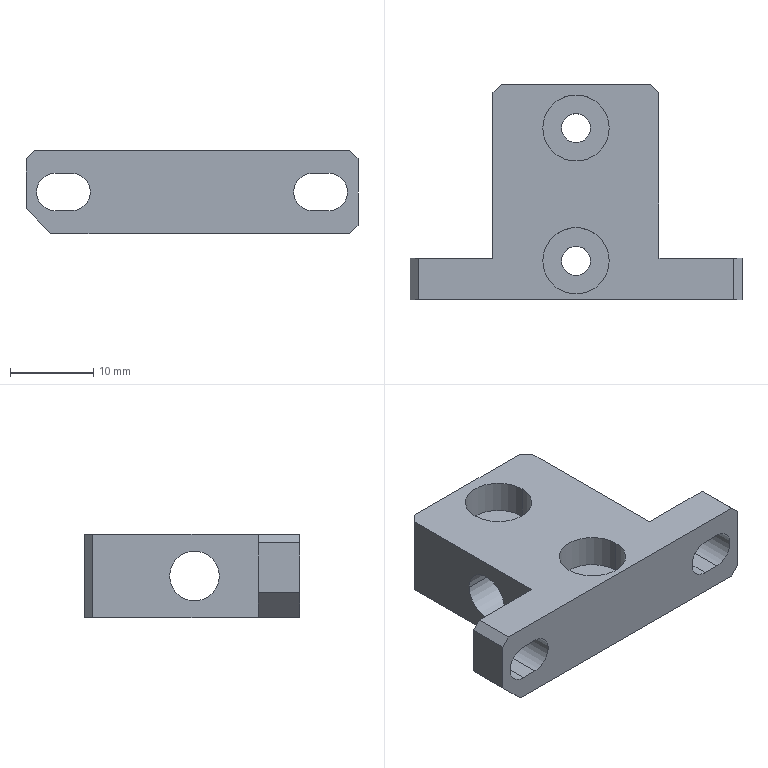Part | SolidWorks | features ICE 3, Chamfer 2, Extrusion 1, HoleWzd 1, MoveFace 1 | 1 solid | 36 faces | box 40 x 26 x 10 mm | volume 4828 mm3 | plane 22 | cylinder 14 | commonest cylinder face diameters 3.5 x4 4.5 x4 8 x4 6 x2
STEP:
#1=CARTESIAN_POINT('',(6.,20.7,6.));
#2=VERTEX_POINT('',#1);
#3=CARTESIAN_POINT('',(14.,20.7,6.));
#4=VERTEX_POINT('',#3);
#5=CARTESIAN_POINT('',(10.,20.7,6.));
#6=DIRECTION('',(0.,0.,1.));
#7=DIRECTION('',(1.,0.,0.));
#8=AXIS2_PLACEMENT_3D('',#5,#6,#7);
#9=CIRCLE('',#8,4.);
#10=EDGE_CURVE('',#2,#4,#9,.T.);
#11=ORIENTED_EDGE('',*,*,#10,.F.);
#12=CARTESIAN_POINT('',(6.,20.7,10.));
#13=VERTEX_POINT('',#12);
#14=CARTESIAN_POINT('',(6.,20.7,10.));
#15=DIRECTION('',(0.,0.,1.));
#16=VECTOR('',#15,1000.);
#17=LINE('',#14,#16);
#18=EDGE_CURVE('',#2,#13,#17,.T.);
#19=ORIENTED_EDGE('',*,*,#18,.T.);
#20=CARTESIAN_POINT('',(14.,20.7,10.));
#21=VERTEX_POINT('',#20);
#22=CARTESIAN_POINT('',(10.,20.7,10.));
#23=DIRECTION('',(0.,0.,1.));
#24=DIRECTION('',(1.,0.,0.));
#25=AXIS2_PLACEMENT_3D('',#22,#23,#24);
#26=CIRCLE('',#25,4.);
#27=EDGE_CURVE('',#13,#21,#26,.T.);
#28=ORIENTED_EDGE('',*,*,#27,.T.);
#29=CARTESIAN_POINT('',(14.,20.7,10.));
#30=DIRECTION('',(0.,0.,1.));
#31=VECTOR('',#30,1000.);
#32=LINE('',#29,#31);
#33=EDGE_CURVE('',#4,#21,#32,.T.);
#34=ORIENTED_EDGE('',*,*,#33,.F.);
#35=EDGE_LOOP('',(#11,#19,#28,#34));
#36=FACE_OUTER_BOUND('',#35,.T.);
#37=CARTESIAN_POINT('',(10.,20.7,10.));
#38=DIRECTION('',(0.,0.,1.));
#39=DIRECTION('',(1.,0.,0.));
#40=AXIS2_PLACEMENT_3D('',#37,#38,#39);
#41=CYLINDRICAL_SURFACE('',#40,4.);
#42=ADVANCED_FACE('',(#36),#41,.F.);
#43=CARTESIAN_POINT('',(11.75,20.7,0.));
#44=VERTEX_POINT('',#43);
#45=CARTESIAN_POINT('',(8.25,20.7,0.));
#46=VERTEX_POINT('',#45);
#47=CARTESIAN_POINT('',(10.,20.7,0.));
#48=DIRECTION('',(0.,0.,-1.));
#49=DIRECTION('',(-1.,0.,0.));
#50=AXIS2_PLACEMENT_3D('',#47,#48,#49);
#51=CIRCLE('',#50,1.75);
#52=EDGE_CURVE('',#44,#46,#51,.T.);
#53=ORIENTED_EDGE('',*,*,#52,.T.);
#54=CARTESIAN_POINT('',(8.25,20.7,6.));
#55=VERTEX_POINT('',#54);
#56=CARTESIAN_POINT('',(8.25,20.7,10.));
#57=DIRECTION('',(0.,0.,1.));
#58=VECTOR('',#57,1000.);
#59=LINE('',#56,#58);
#60=EDGE_CURVE('',#46,#55,#59,.T.);
#61=ORIENTED_EDGE('',*,*,#60,.T.);
#62=CARTESIAN_POINT('',(11.75,20.7,6.));
#63=VERTEX_POINT('',#62);
#64=CARTESIAN_POINT('',(10.,20.7,6.));
#65=DIRECTION('',(0.,0.,1.));
#66=DIRECTION('',(1.,0.,0.));
#67=AXIS2_PLACEMENT_3D('',#64,#65,#66);
#68=CIRCLE('',#67,1.75);
#69=EDGE_CURVE('',#55,#63,#68,.T.);
#70=ORIENTED_EDGE('',*,*,#69,.T.);
#71=CARTESIAN_POINT('',(11.75,20.7,10.));
#72=DIRECTION('',(0.,0.,1.));
#73=VECTOR('',#72,1000.);
#74=LINE('',#71,#73);
#75=EDGE_CURVE('',#44,#63,#74,.T.);
#76=ORIENTED_EDGE('',*,*,#75,.F.);
#77=EDGE_LOOP('',(#53,#61,#70,#76));
#78=FACE_OUTER_BOUND('',#77,.T.);
#79=CARTESIAN_POINT('',(10.,20.7,10.));
#80=DIRECTION('',(0.,0.,1.));
#81=DIRECTION('',(1.,0.,0.));
#82=AXIS2_PLACEMENT_3D('',#79,#80,#81);
#83=CYLINDRICAL_SURFACE('',#82,1.75);
#84=ADVANCED_FACE('',(#78),#83,.F.);
#85=CARTESIAN_POINT('',(6.,4.7,6.));
#86=VERTEX_POINT('',#85);
#87=CARTESIAN_POINT('',(14.,4.7,6.));
#88=VERTEX_POINT('',#87);
#89=CARTESIAN_POINT('',(10.,4.7,6.));
#90=DIRECTION('',(0.,0.,1.));
#91=DIRECTION('',(1.,0.,0.));
#92=AXIS2_PLACEMENT_3D('',#89,#90,#91);
#93=CIRCLE('',#92,4.);
#94=EDGE_CURVE('',#86,#88,#93,.T.);
#95=ORIENTED_EDGE('',*,*,#94,.F.);
#96=CARTESIAN_POINT('',(6.,4.7,10.));
#97=VERTEX_POINT('',#96);
#98=CARTESIAN_POINT('',(6.,4.7,10.));
#99=DIRECTION('',(0.,0.,1.));
#100=VECTOR('',#99,1000.);
#101=LINE('',#98,#100);
#102=EDGE_CURVE('',#86,#97,#101,.T.);
#103=ORIENTED_EDGE('',*,*,#102,.T.);
#104=CARTESIAN_POINT('',(14.,4.7,10.));
#105=VERTEX_POINT('',#104);
#106=CARTESIAN_POINT('',(10.,4.7,10.));
#107=DIRECTION('',(0.,0.,1.));
#108=DIRECTION('',(1.,0.,0.));
#109=AXIS2_PLACEMENT_3D('',#106,#107,#108);
#110=CIRCLE('',#109,4.);
#111=EDGE_CURVE('',#97,#105,#110,.T.);
#112=ORIENTED_EDGE('',*,*,#111,.T.);
#113=CARTESIAN_POINT('',(14.,4.7,10.));
#114=DIRECTION('',(0.,0.,1.));
#115=VECTOR('',#114,1000.);
#116=LINE('',#113,#115);
#117=EDGE_CURVE('',#88,#105,#116,.T.);
#118=ORIENTED_EDGE('',*,*,#117,.F.);
#119=EDGE_LOOP('',(#95,#103,#112,#118));
#120=FACE_OUTER_BOUND('',#119,.T.);
#121=CARTESIAN_POINT('',(10.,4.7,10.));
#122=DIRECTION('',(0.,0.,1.));
#123=DIRECTION('',(1.,0.,0.));
#124=AXIS2_PLACEMENT_3D('',#121,#122,#123);
#125=CYLINDRICAL_SURFACE('',#124,4.);
#126=ADVANCED_FACE('',(#120),#125,.F.);
#127=CARTESIAN_POINT('',(11.75,4.7,0.));
#128=VERTEX_POINT('',#127);
#129=CARTESIAN_POINT('',(8.25,4.7,0.));
#130=VERTEX_POINT('',#129);
#131=CARTESIAN_POINT('',(10.,4.7,0.));
#132=DIRECTION('',(0.,0.,-1.));
#133=DIRECTION('',(-1.,0.,0.));
#134=AXIS2_PLACEMENT_3D('',#131,#132,#133);
#135=CIRCLE('',#134,1.75);
#136=EDGE_CURVE('',#128,#130,#135,.T.);
#137=ORIENTED_EDGE('',*,*,#136,.T.);
#138=CARTESIAN_POINT('',(8.25,4.7,6.));
#139=VERTEX_POINT('',#138);
#140=CARTESIAN_POINT('',(8.25,4.7,10.));
#141=DIRECTION('',(0.,0.,1.));
#142=VECTOR('',#141,1000.);
#143=LINE('',#140,#142);
#144=EDGE_CURVE('',#130,#139,#143,.T.);
#145=ORIENTED_EDGE('',*,*,#144,.T.);
#146=CARTESIAN_POINT('',(11.75,4.7,6.));
#147=VERTEX_POINT('',#146);
#148=CARTESIAN_POINT('',(10.,4.7,6.));
#149=DIRECTION('',(0.,0.,1.));
#150=DIRECTION('',(1.,0.,0.));
#151=AXIS2_PLACEMENT_3D('',#148,#149,#150);
#152=CIRCLE('',#151,1.75);
#153=EDGE_CURVE('',#139,#147,#152,.T.);
#154=ORIENTED_EDGE('',*,*,#153,.T.);
#155=CARTESIAN_POINT('',(11.75,4.7,10.));
#156=DIRECTION('',(0.,0.,1.));
#157=VECTOR('',#156,1000.);
#158=LINE('',#155,#157);
#159=EDGE_CURVE('',#128,#147,#158,.T.);
#160=ORIENTED_EDGE('',*,*,#159,.F.);
#161=EDGE_LOOP('',(#137,#145,#154,#160));
#162=FACE_OUTER_BOUND('',#161,.T.);
#163=CARTESIAN_POINT('',(10.,4.7,10.));
#164=DIRECTION('',(0.,0.,1.));
#165=DIRECTION('',(1.,0.,0.));
#166=AXIS2_PLACEMENT_3D('',#163,#164,#165);
#167=CYLINDRICAL_SURFACE('',#166,1.75);
#168=ADVANCED_FACE('',(#162),#167,.F.);
#169=CARTESIAN_POINT('',(20.,15.7,5.));
#170=VERTEX_POINT('',#169);
#171=CARTESIAN_POINT('',(20.,9.7,5.));
#172=VERTEX_POINT('',#171);
#173=CARTESIAN_POINT('',(20.,12.7,5.));
#174=DIRECTION('',(-1.,0.,0.));
#175=DIRECTION('',(0.,-1.,0.));
#176=AXIS2_PLACEMENT_3D('',#173,#174,#175);
#177=CIRCLE('',#176,3.);
#178=EDGE_CURVE('',#170,#172,#177,.T.);
#179=ORIENTED_EDGE('',*,*,#178,.F.);
#180=CARTESIAN_POINT('',(0.,15.7,5.));
#181=VERTEX_POINT('',#180);
#182=CARTESIAN_POINT('',(30.,15.7,5.));
#183=DIRECTION('',(-1.,0.,0.));
#184=VECTOR('',#183,1000.);
#185=LINE('',#182,#184);
#186=EDGE_CURVE('',#170,#181,#185,.T.);
#187=ORIENTED_EDGE('',*,*,#186,.T.);
#188=CARTESIAN_POINT('',(0.,9.7,5.));
#189=VERTEX_POINT('',#188);
#190=CARTESIAN_POINT('',(0.,12.7,5.));
#191=DIRECTION('',(1.,0.,0.));
#192=DIRECTION('',(0.,0.,-1.));
#193=AXIS2_PLACEMENT_3D('',#190,#191,#192);
#194=CIRCLE('',#193,3.);
#195=EDGE_CURVE('',#189,#181,#194,.T.);
#196=ORIENTED_EDGE('',*,*,#195,.F.);
#197=CARTESIAN_POINT('',(30.,9.7,5.));
#198=DIRECTION('',(-1.,0.,0.));
#199=VECTOR('',#198,1000.);
#200=LINE('',#197,#199);
#201=EDGE_CURVE('',#172,#189,#200,.T.);
#202=ORIENTED_EDGE('',*,*,#201,.F.);
#203=EDGE_LOOP('',(#179,#187,#196,#202));
#204=FACE_OUTER_BOUND('',#203,.T.);
#205=CARTESIAN_POINT('',(30.,12.7,5.));
#206=DIRECTION('',(-1.,0.,0.));
#207=DIRECTION('',(0.,-1.,0.));
#208=AXIS2_PLACEMENT_3D('',#205,#206,#207);
#209=CYLINDRICAL_SURFACE('',#208,3.);
#210=ADVANCED_FACE('',(#204),#209,.F.);
#211=ORIENTED_EDGE('',*,*,#195,.T.);
#212=CARTESIAN_POINT('',(0.,12.7,5.));
#213=DIRECTION('',(1.,0.,0.));
#214=DIRECTION('',(0.,0.,-1.));
#215=AXIS2_PLACEMENT_3D('',#212,#213,#214);
#216=CIRCLE('',#215,3.);
#217=EDGE_CURVE('',#181,#189,#216,.T.);
#218=ORIENTED_EDGE('',*,*,#217,.T.);
#219=EDGE_LOOP('',(#211,#218));
#220=FACE_BOUND('',#219,.T.);
#221=CARTESIAN_POINT('',(0.,25.,10.));
#222=VERTEX_POINT('',#221);
#223=CARTESIAN_POINT('',(0.,5.,10.));
#224=VERTEX_POINT('',#223);
#225=CARTESIAN_POINT('',(0.,0.,10.));
#226=DIRECTION('',(0.,-1.,0.));
#227=VECTOR('',#226,1000.);
#228=LINE('',#225,#227);
#229=EDGE_CURVE('',#222,#224,#228,.T.);
#230=ORIENTED_EDGE('',*,*,#229,.F.);
#231=CARTESIAN_POINT('',(0.,25.,0.));
#232=VERTEX_POINT('',#231);
#233=CARTESIAN_POINT('',(0.,25.,10.));
#234=DIRECTION('',(0.,0.,-1.));
#235=VECTOR('',#234,1000.);
#236=LINE('',#233,#235);
#237=EDGE_CURVE('',#222,#232,#236,.T.);
#238=ORIENTED_EDGE('',*,*,#237,.T.);
#239=CARTESIAN_POINT('',(0.,5.,0.));
#240=VERTEX_POINT('',#239);
#241=CARTESIAN_POINT('',(0.,0.,0.));
#242=DIRECTION('',(0.,-1.,0.));
#243=VECTOR('',#242,1000.);
#244=LINE('',#241,#243);
#245=EDGE_CURVE('',#232,#240,#244,.T.);
#246=ORIENTED_EDGE('',*,*,#245,.T.);
#247=CARTESIAN_POINT('',(0.,5.,10.));
#248=DIRECTION('',(0.,0.,1.));
#249=VECTOR('',#248,1000.);
#250=LINE('',#247,#249);
#251=EDGE_CURVE('',#240,#224,#250,.T.);
#252=ORIENTED_EDGE('',*,*,#251,.T.);
#253=EDGE_LOOP('',(#230,#238,#246,#252));
#254=FACE_OUTER_BOUND('',#253,.T.);
#255=CARTESIAN_POINT('',(0.,0.,10.));
#256=DIRECTION('',(1.,0.,0.));
#257=DIRECTION('',(0.,0.,-1.));
#258=AXIS2_PLACEMENT_3D('',#255,#256,#257);
#259=PLANE('',#258);
#260=ADVANCED_FACE('',(#220,#254),#259,.F.);
#261=CARTESIAN_POINT('',(-4.5,0.,2.75));
#262=VERTEX_POINT('',#261);
#263=CARTESIAN_POINT('',(-6.5,0.,2.75));
#264=VERTEX_POINT('',#263);
#265=CARTESIAN_POINT('',(-6.5,0.,2.75));
#266=DIRECTION('',(-1.,0.,0.));
#267=VECTOR('',#266,1000.);
#268=LINE('',#265,#267);
#269=EDGE_CURVE('',#262,#264,#268,.T.);
#270=ORIENTED_EDGE('',*,*,#269,.T.);
#271=CARTESIAN_POINT('',(-6.5,0.,7.25));
#272=VERTEX_POINT('',#271);
#273=CARTESIAN_POINT('',(-6.5,0.,5.));
#274=DIRECTION('',(0.,1.,0.));
#275=DIRECTION('',(0.,0.,1.));
#276=AXIS2_PLACEMENT_3D('',#273,#274,#275);
#277=CIRCLE('',#276,2.25);
#278=EDGE_CURVE('',#264,#272,#277,.T.);
#279=ORIENTED_EDGE('',*,*,#278,.T.);
#280=CARTESIAN_POINT('',(-4.5,0.,7.25));
#281=VERTEX_POINT('',#280);
#282=CARTESIAN_POINT('',(-6.5,0.,7.25));
#283=DIRECTION('',(1.,0.,0.));
#284=VECTOR('',#283,1000.);
#285=LINE('',#282,#284);
#286=EDGE_CURVE('',#272,#281,#285,.T.);
#287=ORIENTED_EDGE('',*,*,#286,.T.);
#288=CARTESIAN_POINT('',(-4.5,0.,5.));
#289=DIRECTION('',(0.,1.,0.));
#290=DIRECTION('',(0.,0.,1.));
#291=AXIS2_PLACEMENT_3D('',#288,#289,#290);
#292=CIRCLE('',#291,2.25);
#293=EDGE_CURVE('',#281,#262,#292,.T.);
#294=ORIENTED_EDGE('',*,*,#293,.T.);
#295=EDGE_LOOP('',(#270,#279,#287,#294));
#296=FACE_BOUND('',#295,.T.);
#297=CARTESIAN_POINT('',(24.5,0.,7.25));
#298=VERTEX_POINT('',#297);
#299=CARTESIAN_POINT('',(26.5,0.,7.25));
#300=VERTEX_POINT('',#299);
#301=CARTESIAN_POINT('',(26.5,0.,7.25));
#302=DIRECTION('',(1.,0.,0.));
#303=VECTOR('',#302,1000.);
#304=LINE('',#301,#303);
#305=EDGE_CURVE('',#298,#300,#304,.T.);
#306=ORIENTED_EDGE('',*,*,#305,.T.);
#307=CARTESIAN_POINT('',(26.5,0.,2.75));
#308=VERTEX_POINT('',#307);
#309=CARTESIAN_POINT('',(26.5,0.,5.));
#310=DIRECTION('',(0.,1.,0.));
#311=DIRECTION('',(0.,0.,-1.));
#312=AXIS2_PLACEMENT_3D('',#309,#310,#311);
#313=CIRCLE('',#312,2.25);
#314=EDGE_CURVE('',#300,#308,#313,.T.);
#315=ORIENTED_EDGE('',*,*,#314,.T.);
#316=CARTESIAN_POINT('',(24.5,0.,2.75));
#317=VERTEX_POINT('',#316);
#318=CARTESIAN_POINT('',(26.5,0.,2.75));
#319=DIRECTION('',(-1.,0.,0.));
#320=VECTOR('',#319,1000.);
#321=LINE('',#318,#320);
#322=EDGE_CURVE('',#308,#317,#321,.T.);
#323=ORIENTED_EDGE('',*,*,#322,.T.);
#324=CARTESIAN_POINT('',(24.5,0.,5.));
#325=DIRECTION('',(0.,1.,0.));
#326=DIRECTION('',(0.,0.,-1.));
#327=AXIS2_PLACEMENT_3D('',#324,#325,#326);
#328=CIRCLE('',#327,2.25);
#329=EDGE_CURVE('',#317,#298,#328,.T.);
#330=ORIENTED_EDGE('',*,*,#329,.T.);
#331=EDGE_LOOP('',(#306,#315,#323,#330));
#332=FACE_BOUND('',#331,.T.);
#333=CARTESIAN_POINT('',(-10.,0.,9.));
#334=VERTEX_POINT('',#333);
#335=CARTESIAN_POINT('',(-10.,0.,3.));
#336=VERTEX_POINT('',#335);
#337=CARTESIAN_POINT('',(-10.,0.,10.));
#338=DIRECTION('',(0.,0.,-1.));
#339=VECTOR('',#338,1000.);
#340=LINE('',#337,#339);
#341=EDGE_CURVE('',#334,#336,#340,.T.);
#342=ORIENTED_EDGE('',*,*,#341,.T.);
#343=CARTESIAN_POINT('',(-7.,0.,0.));
#344=VERTEX_POINT('',#343);
#345=CARTESIAN_POINT('',(-10.,0.,3.));
#346=DIRECTION('',(0.7071,0.,-0.7071));
#347=VECTOR('',#346,1000.);
#348=LINE('',#345,#347);
#349=EDGE_CURVE('',#336,#344,#348,.T.);
#350=ORIENTED_EDGE('',*,*,#349,.T.);
#351=CARTESIAN_POINT('',(29.,0.,0.));
#352=VERTEX_POINT('',#351);
#353=CARTESIAN_POINT('',(0.,0.,0.));
#354=DIRECTION('',(1.,0.,0.));
#355=VECTOR('',#354,1000.);
#356=LINE('',#353,#355);
#357=EDGE_CURVE('',#344,#352,#356,.T.);
#358=ORIENTED_EDGE('',*,*,#357,.T.);
#359=CARTESIAN_POINT('',(30.,0.,1.));
#360=VERTEX_POINT('',#359);
#361=CARTESIAN_POINT('',(29.,0.,0.));
#362=DIRECTION('',(0.7071,0.,0.7071));
#363=VECTOR('',#362,1000.);
#364=LINE('',#361,#363);
#365=EDGE_CURVE('',#352,#360,#364,.T.);
#366=ORIENTED_EDGE('',*,*,#365,.T.);
#367=CARTESIAN_POINT('',(30.,0.,9.));
#368=VERTEX_POINT('',#367);
#369=CARTESIAN_POINT('',(30.,0.,10.));
#370=DIRECTION('',(0.,0.,1.));
#371=VECTOR('',#370,1000.);
#372=LINE('',#369,#371);
#373=EDGE_CURVE('',#360,#368,#372,.T.);
#374=ORIENTED_EDGE('',*,*,#373,.T.);
#375=CARTESIAN_POINT('',(29.,0.,10.));
#376=VERTEX_POINT('',#375);
#377=CARTESIAN_POINT('',(30.,0.,9.));
#378=DIRECTION('',(-0.7071,0.,0.7071));
#379=VECTOR('',#378,1000.);
#380=LINE('',#377,#379);
#381=EDGE_CURVE('',#368,#376,#380,.T.);
#382=ORIENTED_EDGE('',*,*,#381,.T.);
#383=CARTESIAN_POINT('',(-9.,0.,10.));
#384=VERTEX_POINT('',#383);
#385=CARTESIAN_POINT('',(0.,0.,10.));
#386=DIRECTION('',(1.,0.,0.));
#387=VECTOR('',#386,1000.);
#388=LINE('',#385,#387);
#389=EDGE_CURVE('',#384,#376,#388,.T.);
#390=ORIENTED_EDGE('',*,*,#389,.F.);
#391=CARTESIAN_POINT('',(-9.,0.,10.));
#392=DIRECTION('',(-0.7071,0.,-0.7071));
#393=VECTOR('',#392,1000.);
#394=LINE('',#391,#393);
#395=EDGE_CURVE('',#384,#334,#394,.T.);
#396=ORIENTED_EDGE('',*,*,#395,.T.);
#397=EDGE_LOOP('',(#342,#350,#358,#366,#374,#382,#390,#396));
#398=FACE_OUTER_BOUND('',#397,.T.);
#399=CARTESIAN_POINT('',(0.,0.,10.));
#400=DIRECTION('',(0.,1.,0.));
#401=DIRECTION('',(0.,0.,1.));
#402=AXIS2_PLACEMENT_3D('',#399,#400,#401);
#403=PLANE('',#402);
#404=ADVANCED_FACE('',(#296,#332,#398),#403,.F.);
#405=CARTESIAN_POINT('',(20.,12.7,5.));
#406=DIRECTION('',(-1.,0.,0.));
#407=DIRECTION('',(0.,-1.,0.));
#408=AXIS2_PLACEMENT_3D('',#405,#406,#407);
#409=CIRCLE('',#408,3.);
#410=EDGE_CURVE('',#172,#170,#409,.T.);
#411=ORIENTED_EDGE('',*,*,#410,.T.);
#412=ORIENTED_EDGE('',*,*,#178,.T.);
#413=EDGE_LOOP('',(#411,#412));
#414=FACE_BOUND('',#413,.T.);
#415=CARTESIAN_POINT('',(20.,5.,0.));
#416=VERTEX_POINT('',#415);
#417=CARTESIAN_POINT('',(20.,25.,0.));
#418=VERTEX_POINT('',#417);
#419=CARTESIAN_POINT('',(20.,0.,0.));
#420=DIRECTION('',(0.,1.,0.));
#421=VECTOR('',#420,1000.);
#422=LINE('',#419,#421);
#423=EDGE_CURVE('',#416,#418,#422,.T.);
#424=ORIENTED_EDGE('',*,*,#423,.T.);
#425=CARTESIAN_POINT('',(20.,25.,10.));
#426=VERTEX_POINT('',#425);
#427=CARTESIAN_POINT('',(20.,25.,10.));
#428=DIRECTION('',(0.,0.,1.));
#429=VECTOR('',#428,1000.);
#430=LINE('',#427,#429);
#431=EDGE_CURVE('',#418,#426,#430,.T.);
#432=ORIENTED_EDGE('',*,*,#431,.T.);
#433=CARTESIAN_POINT('',(20.,5.,10.));
#434=VERTEX_POINT('',#433);
#435=CARTESIAN_POINT('',(20.,0.,10.));
#436=DIRECTION('',(0.,1.,0.));
#437=VECTOR('',#436,1000.);
#438=LINE('',#435,#437);
#439=EDGE_CURVE('',#434,#426,#438,.T.);
#440=ORIENTED_EDGE('',*,*,#439,.F.);
#441=CARTESIAN_POINT('',(20.,5.,10.));
#442=DIRECTION('',(0.,0.,-1.));
#443=VECTOR('',#442,1000.);
#444=LINE('',#441,#443);
#445=EDGE_CURVE('',#434,#416,#444,.T.);
#446=ORIENTED_EDGE('',*,*,#445,.T.);
#447=EDGE_LOOP('',(#424,#432,#440,#446));
#448=FACE_OUTER_BOUND('',#447,.T.);
#449=CARTESIAN_POINT('',(20.,0.,10.));
#450=DIRECTION('',(-1.,0.,0.));
#451=DIRECTION('',(0.,-1.,0.));
#452=AXIS2_PLACEMENT_3D('',#449,#450,#451);
#453=PLANE('',#452);
#454=ADVANCED_FACE('',(#414,#448),#453,.F.);
#455=CARTESIAN_POINT('',(19.,26.,10.));
#456=VERTEX_POINT('',#455);
#457=CARTESIAN_POINT('',(1.,26.,10.));
#458=VERTEX_POINT('',#457);
#459=CARTESIAN_POINT('',(0.,26.,10.));
#460=DIRECTION('',(-1.,0.,0.));
#461=VECTOR('',#460,1000.);
#462=LINE('',#459,#461);
#463=EDGE_CURVE('',#456,#458,#462,.T.);
#464=ORIENTED_EDGE('',*,*,#463,.F.);
#465=CARTESIAN_POINT('',(19.,26.,0.));
#466=VERTEX_POINT('',#465);
#467=CARTESIAN_POINT('',(19.,26.,10.));
#468=DIRECTION('',(0.,0.,-1.));
#469=VECTOR('',#468,1000.);
#470=LINE('',#467,#469);
#471=EDGE_CURVE('',#456,#466,#470,.T.);
#472=ORIENTED_EDGE('',*,*,#471,.T.);
#473=CARTESIAN_POINT('',(1.,26.,0.));
#474=VERTEX_POINT('',#473);
#475=CARTESIAN_POINT('',(0.,26.,0.));
#476=DIRECTION('',(-1.,0.,0.));
#477=VECTOR('',#476,1000.);
#478=LINE('',#475,#477);
#479=EDGE_CURVE('',#466,#474,#478,.T.);
#480=ORIENTED_EDGE('',*,*,#479,.T.);
#481=CARTESIAN_POINT('',(1.,26.,10.));
#482=DIRECTION('',(0.,0.,1.));
#483=VECTOR('',#482,1000.);
#484=LINE('',#481,#483);
#485=EDGE_CURVE('',#474,#458,#484,.T.);
#486=ORIENTED_EDGE('',*,*,#485,.T.);
#487=EDGE_LOOP('',(#464,#472,#480,#486));
#488=FACE_OUTER_BOUND('',#487,.T.);
#489=CARTESIAN_POINT('',(0.,26.,10.));
#490=DIRECTION('',(0.,-1.,0.));
#491=DIRECTION('',(0.,0.,-1.));
#492=AXIS2_PLACEMENT_3D('',#489,#490,#491);
#493=PLANE('',#492);
#494=ADVANCED_FACE('',(#488),#493,.F.);
#495=CARTESIAN_POINT('',(10.,20.7,10.));
#496=DIRECTION('',(0.,0.,1.));
#497=DIRECTION('',(1.,0.,0.));
#498=AXIS2_PLACEMENT_3D('',#495,#496,#497);
#499=CIRCLE('',#498,4.);
#500=EDGE_CURVE('',#21,#13,#499,.T.);
#501=ORIENTED_EDGE('',*,*,#500,.F.);
#502=ORIENTED_EDGE('',*,*,#27,.F.);
#503=EDGE_LOOP('',(#501,#502));
#504=FACE_BOUND('',#503,.T.);
#505=CARTESIAN_POINT('',(10.,4.7,10.));
#506=DIRECTION('',(0.,0.,1.));
#507=DIRECTION('',(1.,0.,0.));
#508=AXIS2_PLACEMENT_3D('',#505,#506,#507);
#509=CIRCLE('',#508,4.);
#510=EDGE_CURVE('',#105,#97,#509,.T.);
#511=ORIENTED_EDGE('',*,*,#510,.F.);
#512=ORIENTED_EDGE('',*,*,#111,.F.);
#513=EDGE_LOOP('',(#511,#512));
#514=FACE_BOUND('',#513,.T.);
#515=ORIENTED_EDGE('',*,*,#389,.T.);
#516=CARTESIAN_POINT('',(29.,5.,10.));
#517=VERTEX_POINT('',#516);
#518=CARTESIAN_POINT('',(29.,8.,10.));
#519=DIRECTION('',(0.,1.,0.));
#520=VECTOR('',#519,1000.);
#521=LINE('',#518,#520);
#522=EDGE_CURVE('',#376,#517,#521,.T.);
#523=ORIENTED_EDGE('',*,*,#522,.T.);
#524=CARTESIAN_POINT('',(-10.,5.,10.));
#525=DIRECTION('',(-1.,0.,0.));
#526=VECTOR('',#525,1000.);
#527=LINE('',#524,#526);
#528=EDGE_CURVE('',#517,#434,#527,.T.);
#529=ORIENTED_EDGE('',*,*,#528,.T.);
#530=ORIENTED_EDGE('',*,*,#439,.T.);
#531=CARTESIAN_POINT('',(19.,26.,10.));
#532=DIRECTION('',(-0.7071,0.7071,0.));
#533=VECTOR('',#532,1000.);
#534=LINE('',#531,#533);
#535=EDGE_CURVE('',#426,#456,#534,.T.);
#536=ORIENTED_EDGE('',*,*,#535,.T.);
#537=ORIENTED_EDGE('',*,*,#463,.T.);
#538=CARTESIAN_POINT('',(0.,25.,10.));
#539=DIRECTION('',(-0.7071,-0.7071,0.));
#540=VECTOR('',#539,1000.);
#541=LINE('',#538,#540);
#542=EDGE_CURVE('',#458,#222,#541,.T.);
#543=ORIENTED_EDGE('',*,*,#542,.T.);
#544=ORIENTED_EDGE('',*,*,#229,.T.);
#545=CARTESIAN_POINT('',(-9.,5.,10.));
#546=VERTEX_POINT('',#545);
#547=CARTESIAN_POINT('',(-10.,5.,10.));
#548=DIRECTION('',(-1.,0.,0.));
#549=VECTOR('',#548,1000.);
#550=LINE('',#547,#549);
#551=EDGE_CURVE('',#224,#546,#550,.T.);
#552=ORIENTED_EDGE('',*,*,#551,.T.);
#553=CARTESIAN_POINT('',(-9.,0.,10.));
#554=DIRECTION('',(0.,-1.,0.));
#555=VECTOR('',#554,1000.);
#556=LINE('',#553,#555);
#557=EDGE_CURVE('',#546,#384,#556,.T.);
#558=ORIENTED_EDGE('',*,*,#557,.T.);
#559=EDGE_LOOP('',(#515,#523,#529,#530,#536,#537,#543,#544,#552,#558));
#560=FACE_OUTER_BOUND('',#559,.T.);
#561=CARTESIAN_POINT('',(0.,0.,10.));
#562=DIRECTION('',(0.,0.,-1.));
#563=DIRECTION('',(-1.,0.,0.));
#564=AXIS2_PLACEMENT_3D('',#561,#562,#563);
#565=PLANE('',#564);
#566=ADVANCED_FACE('',(#504,#514,#560),#565,.F.);
#567=ORIENTED_EDGE('',*,*,#52,.F.);
#568=CARTESIAN_POINT('',(10.,20.7,0.));
#569=DIRECTION('',(0.,0.,-1.));
#570=DIRECTION('',(-1.,0.,0.));
#571=AXIS2_PLACEMENT_3D('',#568,#569,#570);
#572=CIRCLE('',#571,1.75);
#573=EDGE_CURVE('',#46,#44,#572,.T.);
#574=ORIENTED_EDGE('',*,*,#573,.F.);
#575=EDGE_LOOP('',(#567,#574));
#576=FACE_BOUND('',#575,.T.);
#577=ORIENTED_EDGE('',*,*,#136,.F.);
#578=CARTESIAN_POINT('',(10.,4.7,0.));
#579=DIRECTION('',(0.,0.,-1.));
#580=DIRECTION('',(-1.,0.,0.));
#581=AXIS2_PLACEMENT_3D('',#578,#579,#580);
#582=CIRCLE('',#581,1.75);
#583=EDGE_CURVE('',#130,#128,#582,.T.);
#584=ORIENTED_EDGE('',*,*,#583,.F.);
#585=EDGE_LOOP('',(#577,#584));
#586=FACE_BOUND('',#585,.T.);
#587=ORIENTED_EDGE('',*,*,#357,.F.);
#588=CARTESIAN_POINT('',(-7.,5.,0.));
#589=VERTEX_POINT('',#588);
#590=CARTESIAN_POINT('',(-7.,0.,0.));
#591=DIRECTION('',(0.,1.,0.));
#592=VECTOR('',#591,1000.);
#593=LINE('',#590,#592);
#594=EDGE_CURVE('',#344,#589,#593,.T.);
#595=ORIENTED_EDGE('',*,*,#594,.T.);
#596=CARTESIAN_POINT('',(-10.,5.,0.));
#597=DIRECTION('',(1.,0.,0.));
#598=VECTOR('',#597,1000.);
#599=LINE('',#596,#598);
#600=EDGE_CURVE('',#589,#240,#599,.T.);
#601=ORIENTED_EDGE('',*,*,#600,.T.);
#602=ORIENTED_EDGE('',*,*,#245,.F.);
#603=CARTESIAN_POINT('',(-12.5,12.5,0.));
#604=DIRECTION('',(0.7071,0.7071,0.));
#605=VECTOR('',#604,1000.);
#606=LINE('',#603,#605);
#607=EDGE_CURVE('',#232,#474,#606,.T.);
#608=ORIENTED_EDGE('',*,*,#607,.T.);
#609=ORIENTED_EDGE('',*,*,#479,.F.);
#610=CARTESIAN_POINT('',(22.5,22.5,0.));
#611=DIRECTION('',(0.7071,-0.7071,0.));
#612=VECTOR('',#611,1000.);
#613=LINE('',#610,#612);
#614=EDGE_CURVE('',#466,#418,#613,.T.);
#615=ORIENTED_EDGE('',*,*,#614,.T.);
#616=ORIENTED_EDGE('',*,*,#423,.F.);
#617=CARTESIAN_POINT('',(29.,5.,0.));
#618=VERTEX_POINT('',#617);
#619=CARTESIAN_POINT('',(-10.,5.,0.));
#620=DIRECTION('',(1.,0.,0.));
#621=VECTOR('',#620,1000.);
#622=LINE('',#619,#621);
#623=EDGE_CURVE('',#416,#618,#622,.T.);
#624=ORIENTED_EDGE('',*,*,#623,.T.);
#625=CARTESIAN_POINT('',(29.,0.,0.));
#626=DIRECTION('',(0.,-1.,0.));
#627=VECTOR('',#626,1000.);
#628=LINE('',#625,#627);
#629=EDGE_CURVE('',#618,#352,#628,.T.);
#630=ORIENTED_EDGE('',*,*,#629,.T.);
#631=EDGE_LOOP('',(#587,#595,#601,#602,#608,#609,#615,#616,#624,#630));
#632=FACE_OUTER_BOUND('',#631,.T.);
#633=CARTESIAN_POINT('',(0.,0.,0.));
#634=DIRECTION('',(0.,0.,-1.));
#635=DIRECTION('',(-1.,0.,0.));
#636=AXIS2_PLACEMENT_3D('',#633,#634,#635);
#637=PLANE('',#636);
#638=ADVANCED_FACE('',(#576,#586,#632),#637,.T.);
#639=ORIENTED_EDGE('',*,*,#373,.F.);
#640=CARTESIAN_POINT('',(30.,5.,1.));
#641=VERTEX_POINT('',#640);
#642=CARTESIAN_POINT('',(30.,8.,1.));
#643=DIRECTION('',(0.,1.,0.));
#644=VECTOR('',#643,1000.);
#645=LINE('',#642,#644);
#646=EDGE_CURVE('',#360,#641,#645,.T.);
#647=ORIENTED_EDGE('',*,*,#646,.T.);
#648=CARTESIAN_POINT('',(30.,5.,9.));
#649=VERTEX_POINT('',#648);
#650=CARTESIAN_POINT('',(30.,5.,10.));
#651=DIRECTION('',(0.,0.,1.));
#652=VECTOR('',#651,1000.);
#653=LINE('',#650,#652);
#654=EDGE_CURVE('',#641,#649,#653,.T.);
#655=ORIENTED_EDGE('',*,*,#654,.T.);
#656=CARTESIAN_POINT('',(30.,0.,9.));
#657=DIRECTION('',(0.,-1.,0.));
#658=VECTOR('',#657,1000.);
#659=LINE('',#656,#658);
#660=EDGE_CURVE('',#649,#368,#659,.T.);
#661=ORIENTED_EDGE('',*,*,#660,.T.);
#662=EDGE_LOOP('',(#639,#647,#655,#661));
#663=FACE_OUTER_BOUND('',#662,.T.);
#664=CARTESIAN_POINT('',(30.,8.,10.));
#665=DIRECTION('',(1.,0.,0.));
#666=DIRECTION('',(0.,0.,-1.));
#667=AXIS2_PLACEMENT_3D('',#664,#665,#666);
#668=PLANE('',#667);
#669=ADVANCED_FACE('',(#663),#668,.T.);
#670=CARTESIAN_POINT('',(26.5,5.,7.25));
#671=VERTEX_POINT('',#670);
#672=CARTESIAN_POINT('',(26.5,5.,2.75));
#673=VERTEX_POINT('',#672);
#674=CARTESIAN_POINT('',(26.5,5.,5.));
#675=DIRECTION('',(0.,1.,0.));
#676=DIRECTION('',(0.,0.,-1.));
#677=AXIS2_PLACEMENT_3D('',#674,#675,#676);
#678=CIRCLE('',#677,2.25);
#679=EDGE_CURVE('',#671,#673,#678,.T.);
#680=ORIENTED_EDGE('',*,*,#679,.F.);
#681=CARTESIAN_POINT('',(24.5,5.,7.25));
#682=VERTEX_POINT('',#681);
#683=CARTESIAN_POINT('',(26.5,5.,7.25));
#684=DIRECTION('',(1.,0.,0.));
#685=VECTOR('',#684,1000.);
#686=LINE('',#683,#685);
#687=EDGE_CURVE('',#682,#671,#686,.T.);
#688=ORIENTED_EDGE('',*,*,#687,.F.);
#689=CARTESIAN_POINT('',(24.5,5.,2.75));
#690=VERTEX_POINT('',#689);
#691=CARTESIAN_POINT('',(24.5,5.,5.));
#692=DIRECTION('',(0.,1.,0.));
#693=DIRECTION('',(0.,0.,-1.));
#694=AXIS2_PLACEMENT_3D('',#691,#692,#693);
#695=CIRCLE('',#694,2.25);
#696=EDGE_CURVE('',#690,#682,#695,.T.);
#697=ORIENTED_EDGE('',*,*,#696,.F.);
#698=CARTESIAN_POINT('',(26.5,5.,2.75));
#699=DIRECTION('',(-1.,0.,0.));
#700=VECTOR('',#699,1000.);
#701=LINE('',#698,#700);
#702=EDGE_CURVE('',#673,#690,#701,.T.);
#703=ORIENTED_EDGE('',*,*,#702,.F.);
#704=EDGE_LOOP('',(#680,#688,#697,#703));
#705=FACE_BOUND('',#704,.T.);
#706=ORIENTED_EDGE('',*,*,#654,.F.);
#707=CARTESIAN_POINT('',(14.5,5.,-14.5));
#708=DIRECTION('',(-0.7071,0.,-0.7071));
#709=VECTOR('',#708,1000.);
#710=LINE('',#707,#709);
#711=EDGE_CURVE('',#641,#618,#710,.T.);
#712=ORIENTED_EDGE('',*,*,#711,.T.);
#713=ORIENTED_EDGE('',*,*,#623,.F.);
#714=ORIENTED_EDGE('',*,*,#445,.F.);
#715=ORIENTED_EDGE('',*,*,#528,.F.);
#716=CARTESIAN_POINT('',(19.5,5.,19.5));
#717=DIRECTION('',(0.7071,0.,-0.7071));
#718=VECTOR('',#717,1000.);
#719=LINE('',#716,#718);
#720=EDGE_CURVE('',#517,#649,#719,.T.);
#721=ORIENTED_EDGE('',*,*,#720,.T.);
#722=EDGE_LOOP('',(#706,#712,#713,#714,#715,#721));
#723=FACE_OUTER_BOUND('',#722,.T.);
#724=CARTESIAN_POINT('',(0.,5.,0.));
#725=DIRECTION('',(0.,1.,0.));
#726=DIRECTION('',(0.,0.,1.));
#727=AXIS2_PLACEMENT_3D('',#724,#725,#726);
#728=PLANE('',#727);
#729=ADVANCED_FACE('',(#705,#723),#728,.T.);
#730=CARTESIAN_POINT('',(-6.5,5.,2.75));
#731=VERTEX_POINT('',#730);
#732=CARTESIAN_POINT('',(-6.5,5.,7.25));
#733=VERTEX_POINT('',#732);
#734=CARTESIAN_POINT('',(-6.5,5.,5.));
#735=DIRECTION('',(0.,1.,0.));
#736=DIRECTION('',(0.,0.,1.));
#737=AXIS2_PLACEMENT_3D('',#734,#735,#736);
#738=CIRCLE('',#737,2.25);
#739=EDGE_CURVE('',#731,#733,#738,.T.);
#740=ORIENTED_EDGE('',*,*,#739,.F.);
#741=CARTESIAN_POINT('',(-4.5,5.,2.75));
#742=VERTEX_POINT('',#741);
#743=CARTESIAN_POINT('',(-6.5,5.,2.75));
#744=DIRECTION('',(-1.,0.,0.));
#745=VECTOR('',#744,1000.);
#746=LINE('',#743,#745);
#747=EDGE_CURVE('',#742,#731,#746,.T.);
#748=ORIENTED_EDGE('',*,*,#747,.F.);
#749=CARTESIAN_POINT('',(-4.5,5.,7.25));
#750=VERTEX_POINT('',#749);
#751=CARTESIAN_POINT('',(-4.5,5.,5.));
#752=DIRECTION('',(0.,1.,0.));
#753=DIRECTION('',(0.,0.,1.));
#754=AXIS2_PLACEMENT_3D('',#751,#752,#753);
#755=CIRCLE('',#754,2.25);
#756=EDGE_CURVE('',#750,#742,#755,.T.);
#757=ORIENTED_EDGE('',*,*,#756,.F.);
#758=CARTESIAN_POINT('',(-6.5,5.,7.25));
#759=DIRECTION('',(1.,0.,0.));
#760=VECTOR('',#759,1000.);
#761=LINE('',#758,#760);
#762=EDGE_CURVE('',#733,#750,#761,.T.);
#763=ORIENTED_EDGE('',*,*,#762,.F.);
#764=EDGE_LOOP('',(#740,#748,#757,#763));
#765=FACE_BOUND('',#764,.T.);
#766=ORIENTED_EDGE('',*,*,#600,.F.);
#767=CARTESIAN_POINT('',(-10.,5.,3.));
#768=VERTEX_POINT('',#767);
#769=CARTESIAN_POINT('',(-3.5,5.,-3.5));
#770=DIRECTION('',(-0.7071,0.,0.7071));
#771=VECTOR('',#770,1000.);
#772=LINE('',#769,#771);
#773=EDGE_CURVE('',#589,#768,#772,.T.);
#774=ORIENTED_EDGE('',*,*,#773,.T.);
#775=CARTESIAN_POINT('',(-10.,5.,9.));
#776=VERTEX_POINT('',#775);
#777=CARTESIAN_POINT('',(-10.,5.,10.));
#778=DIRECTION('',(0.,0.,-1.));
#779=VECTOR('',#778,1000.);
#780=LINE('',#777,#779);
#781=EDGE_CURVE('',#776,#768,#780,.T.);
#782=ORIENTED_EDGE('',*,*,#781,.F.);
#783=CARTESIAN_POINT('',(-9.5,5.,9.5));
#784=DIRECTION('',(0.7071,0.,0.7071));
#785=VECTOR('',#784,1000.);
#786=LINE('',#783,#785);
#787=EDGE_CURVE('',#776,#546,#786,.T.);
#788=ORIENTED_EDGE('',*,*,#787,.T.);
#789=ORIENTED_EDGE('',*,*,#551,.F.);
#790=ORIENTED_EDGE('',*,*,#251,.F.);
#791=EDGE_LOOP('',(#766,#774,#782,#788,#789,#790));
#792=FACE_OUTER_BOUND('',#791,.T.);
#793=CARTESIAN_POINT('',(0.,5.,0.));
#794=DIRECTION('',(0.,1.,0.));
#795=DIRECTION('',(0.,0.,1.));
#796=AXIS2_PLACEMENT_3D('',#793,#794,#795);
#797=PLANE('',#796);
#798=ADVANCED_FACE('',(#765,#792),#797,.T.);
#799=ORIENTED_EDGE('',*,*,#781,.T.);
#800=CARTESIAN_POINT('',(-10.,8.,3.));
#801=DIRECTION('',(0.,-1.,0.));
#802=VECTOR('',#801,1000.);
#803=LINE('',#800,#802);
#804=EDGE_CURVE('',#768,#336,#803,.T.);
#805=ORIENTED_EDGE('',*,*,#804,.T.);
#806=ORIENTED_EDGE('',*,*,#341,.F.);
#807=CARTESIAN_POINT('',(-10.,8.,9.));
#808=DIRECTION('',(0.,1.,0.));
#809=VECTOR('',#808,1000.);
#810=LINE('',#807,#809);
#811=EDGE_CURVE('',#334,#776,#810,.T.);
#812=ORIENTED_EDGE('',*,*,#811,.T.);
#813=EDGE_LOOP('',(#799,#805,#806,#812));
#814=FACE_OUTER_BOUND('',#813,.T.);
#815=CARTESIAN_POINT('',(-10.,8.,10.));
#816=DIRECTION('',(-1.,0.,0.));
#817=DIRECTION('',(0.,0.,1.));
#818=AXIS2_PLACEMENT_3D('',#815,#816,#817);
#819=PLANE('',#818);
#820=ADVANCED_FACE('',(#814),#819,.T.);
#821=ORIENTED_EDGE('',*,*,#739,.T.);
#822=CARTESIAN_POINT('',(-6.5,0.,7.25));
#823=DIRECTION('',(0.,1.,0.));
#824=VECTOR('',#823,1000.);
#825=LINE('',#822,#824);
#826=EDGE_CURVE('',#272,#733,#825,.T.);
#827=ORIENTED_EDGE('',*,*,#826,.F.);
#828=ORIENTED_EDGE('',*,*,#278,.F.);
#829=CARTESIAN_POINT('',(-6.5,0.,2.75));
#830=DIRECTION('',(0.,1.,0.));
#831=VECTOR('',#830,1000.);
#832=LINE('',#829,#831);
#833=EDGE_CURVE('',#264,#731,#832,.T.);
#834=ORIENTED_EDGE('',*,*,#833,.T.);
#835=EDGE_LOOP('',(#821,#827,#828,#834));
#836=FACE_OUTER_BOUND('',#835,.T.);
#837=CARTESIAN_POINT('',(-6.5,0.,5.));
#838=DIRECTION('',(0.,1.,0.));
#839=DIRECTION('',(0.,0.,1.));
#840=AXIS2_PLACEMENT_3D('',#837,#838,#839);
#841=CYLINDRICAL_SURFACE('',#840,2.25);
#842=ADVANCED_FACE('',(#836),#841,.F.);
#843=ORIENTED_EDGE('',*,*,#747,.T.);
#844=ORIENTED_EDGE('',*,*,#833,.F.);
#845=ORIENTED_EDGE('',*,*,#269,.F.);
#846=CARTESIAN_POINT('',(-4.5,0.,2.75));
#847=DIRECTION('',(0.,1.,0.));
#848=VECTOR('',#847,1000.);
#849=LINE('',#846,#848);
#850=EDGE_CURVE('',#262,#742,#849,.T.);
#851=ORIENTED_EDGE('',*,*,#850,.T.);
#852=EDGE_LOOP('',(#843,#844,#845,#851));
#853=FACE_OUTER_BOUND('',#852,.T.);
#854=CARTESIAN_POINT('',(-6.5,0.,2.75));
#855=DIRECTION('',(0.,0.,-1.));
#856=DIRECTION('',(-1.,0.,0.));
#857=AXIS2_PLACEMENT_3D('',#854,#855,#856);
#858=PLANE('',#857);
#859=ADVANCED_FACE('',(#853),#858,.F.);
#860=ORIENTED_EDGE('',*,*,#756,.T.);
#861=ORIENTED_EDGE('',*,*,#850,.F.);
#862=ORIENTED_EDGE('',*,*,#293,.F.);
#863=CARTESIAN_POINT('',(-4.5,0.,7.25));
#864=DIRECTION('',(0.,1.,0.));
#865=VECTOR('',#864,1000.);
#866=LINE('',#863,#865);
#867=EDGE_CURVE('',#281,#750,#866,.T.);
#868=ORIENTED_EDGE('',*,*,#867,.T.);
#869=EDGE_LOOP('',(#860,#861,#862,#868));
#870=FACE_OUTER_BOUND('',#869,.T.);
#871=CARTESIAN_POINT('',(-4.5,0.,5.));
#872=DIRECTION('',(0.,1.,0.));
#873=DIRECTION('',(0.,0.,1.));
#874=AXIS2_PLACEMENT_3D('',#871,#872,#873);
#875=CYLINDRICAL_SURFACE('',#874,2.25);
#876=ADVANCED_FACE('',(#870),#875,.F.);
#877=ORIENTED_EDGE('',*,*,#762,.T.);
#878=ORIENTED_EDGE('',*,*,#867,.F.);
#879=ORIENTED_EDGE('',*,*,#286,.F.);
#880=ORIENTED_EDGE('',*,*,#826,.T.);
#881=EDGE_LOOP('',(#877,#878,#879,#880));
#882=FACE_OUTER_BOUND('',#881,.T.);
#883=CARTESIAN_POINT('',(-6.5,0.,7.25));
#884=DIRECTION('',(0.,0.,1.));
#885=DIRECTION('',(1.,0.,0.));
#886=AXIS2_PLACEMENT_3D('',#883,#884,#885);
#887=PLANE('',#886);
#888=ADVANCED_FACE('',(#882),#887,.F.);
#889=ORIENTED_EDGE('',*,*,#679,.T.);
#890=CARTESIAN_POINT('',(26.5,0.,2.75));
#891=DIRECTION('',(0.,1.,0.));
#892=VECTOR('',#891,1000.);
#893=LINE('',#890,#892);
#894=EDGE_CURVE('',#308,#673,#893,.T.);
#895=ORIENTED_EDGE('',*,*,#894,.F.);
#896=ORIENTED_EDGE('',*,*,#314,.F.);
#897=CARTESIAN_POINT('',(26.5,0.,7.25));
#898=DIRECTION('',(0.,1.,0.));
#899=VECTOR('',#898,1000.);
#900=LINE('',#897,#899);
#901=EDGE_CURVE('',#300,#671,#900,.T.);
#902=ORIENTED_EDGE('',*,*,#901,.T.);
#903=EDGE_LOOP('',(#889,#895,#896,#902));
#904=FACE_OUTER_BOUND('',#903,.T.);
#905=CARTESIAN_POINT('',(26.5,0.,5.));
#906=DIRECTION('',(0.,1.,0.));
#907=DIRECTION('',(0.,0.,1.));
#908=AXIS2_PLACEMENT_3D('',#905,#906,#907);
#909=CYLINDRICAL_SURFACE('',#908,2.25);
#910=ADVANCED_FACE('',(#904),#909,.F.);
#911=ORIENTED_EDGE('',*,*,#687,.T.);
#912=ORIENTED_EDGE('',*,*,#901,.F.);
#913=ORIENTED_EDGE('',*,*,#305,.F.);
#914=CARTESIAN_POINT('',(24.5,0.,7.25));
#915=DIRECTION('',(0.,1.,0.));
#916=VECTOR('',#915,1000.);
#917=LINE('',#914,#916);
#918=EDGE_CURVE('',#298,#682,#917,.T.);
#919=ORIENTED_EDGE('',*,*,#918,.T.);
#920=EDGE_LOOP('',(#911,#912,#913,#919));
#921=FACE_OUTER_BOUND('',#920,.T.);
#922=CARTESIAN_POINT('',(26.5,0.,7.25));
#923=DIRECTION('',(0.,0.,1.));
#924=DIRECTION('',(1.,0.,0.));
#925=AXIS2_PLACEMENT_3D('',#922,#923,#924);
#926=PLANE('',#925);
#927=ADVANCED_FACE('',(#921),#926,.F.);
#928=ORIENTED_EDGE('',*,*,#696,.T.);
#929=ORIENTED_EDGE('',*,*,#918,.F.);
#930=ORIENTED_EDGE('',*,*,#329,.F.);
#931=CARTESIAN_POINT('',(24.5,0.,2.75));
#932=DIRECTION('',(0.,1.,0.));
#933=VECTOR('',#932,1000.);
#934=LINE('',#931,#933);
#935=EDGE_CURVE('',#317,#690,#934,.T.);
#936=ORIENTED_EDGE('',*,*,#935,.T.);
#937=EDGE_LOOP('',(#928,#929,#930,#936));
#938=FACE_OUTER_BOUND('',#937,.T.);
#939=CARTESIAN_POINT('',(24.5,0.,5.));
#940=DIRECTION('',(0.,1.,0.));
#941=DIRECTION('',(0.,0.,1.));
#942=AXIS2_PLACEMENT_3D('',#939,#940,#941);
#943=CYLINDRICAL_SURFACE('',#942,2.25);
#944=ADVANCED_FACE('',(#938),#943,.F.);
#945=ORIENTED_EDGE('',*,*,#702,.T.);
#946=ORIENTED_EDGE('',*,*,#935,.F.);
#947=ORIENTED_EDGE('',*,*,#322,.F.);
#948=ORIENTED_EDGE('',*,*,#894,.T.);
#949=EDGE_LOOP('',(#945,#946,#947,#948));
#950=FACE_OUTER_BOUND('',#949,.T.);
#951=CARTESIAN_POINT('',(26.5,0.,2.75));
#952=DIRECTION('',(0.,0.,-1.));
#953=DIRECTION('',(-1.,0.,0.));
#954=AXIS2_PLACEMENT_3D('',#951,#952,#953);
#955=PLANE('',#954);
#956=ADVANCED_FACE('',(#950),#955,.F.);
#957=ORIENTED_EDGE('',*,*,#186,.F.);
#958=ORIENTED_EDGE('',*,*,#410,.F.);
#959=ORIENTED_EDGE('',*,*,#201,.T.);
#960=ORIENTED_EDGE('',*,*,#217,.F.);
#961=EDGE_LOOP('',(#957,#958,#959,#960));
#962=FACE_OUTER_BOUND('',#961,.T.);
#963=CARTESIAN_POINT('',(30.,12.7,5.));
#964=DIRECTION('',(-1.,0.,0.));
#965=DIRECTION('',(0.,-1.,0.));
#966=AXIS2_PLACEMENT_3D('',#963,#964,#965);
#967=CYLINDRICAL_SURFACE('',#966,3.);
#968=ADVANCED_FACE('',(#962),#967,.F.);
#969=ORIENTED_EDGE('',*,*,#144,.F.);
#970=ORIENTED_EDGE('',*,*,#583,.T.);
#971=ORIENTED_EDGE('',*,*,#159,.T.);
#972=CARTESIAN_POINT('',(10.,4.7,6.));
#973=DIRECTION('',(0.,0.,1.));
#974=DIRECTION('',(1.,0.,0.));
#975=AXIS2_PLACEMENT_3D('',#972,#973,#974);
#976=CIRCLE('',#975,1.75);
#977=EDGE_CURVE('',#147,#139,#976,.T.);
#978=ORIENTED_EDGE('',*,*,#977,.T.);
#979=EDGE_LOOP('',(#969,#970,#971,#978));
#980=FACE_OUTER_BOUND('',#979,.T.);
#981=CARTESIAN_POINT('',(10.,4.7,10.));
#982=DIRECTION('',(0.,0.,1.));
#983=DIRECTION('',(1.,0.,0.));
#984=AXIS2_PLACEMENT_3D('',#981,#982,#983);
#985=CYLINDRICAL_SURFACE('',#984,1.75);
#986=ADVANCED_FACE('',(#980),#985,.F.);
#987=ORIENTED_EDGE('',*,*,#977,.F.);
#988=ORIENTED_EDGE('',*,*,#153,.F.);
#989=EDGE_LOOP('',(#987,#988));
#990=FACE_BOUND('',#989,.T.);
#991=CARTESIAN_POINT('',(10.,4.7,6.));
#992=DIRECTION('',(0.,0.,1.));
#993=DIRECTION('',(1.,0.,0.));
#994=AXIS2_PLACEMENT_3D('',#991,#992,#993);
#995=CIRCLE('',#994,4.);
#996=EDGE_CURVE('',#88,#86,#995,.T.);
#997=ORIENTED_EDGE('',*,*,#996,.T.);
#998=ORIENTED_EDGE('',*,*,#94,.T.);
#999=EDGE_LOOP('',(#997,#998));
#1000=FACE_OUTER_BOUND('',#999,.T.);
#1001=CARTESIAN_POINT('',(11.75,4.7,6.));
#1002=DIRECTION('',(0.,0.,-1.));
#1003=DIRECTION('',(-1.,0.,0.));
#1004=AXIS2_PLACEMENT_3D('',#1001,#1002,#1003);
#1005=PLANE('',#1004);
#1006=ADVANCED_FACE('',(#990,#1000),#1005,.F.);
#1007=ORIENTED_EDGE('',*,*,#102,.F.);
#1008=ORIENTED_EDGE('',*,*,#996,.F.);
#1009=ORIENTED_EDGE('',*,*,#117,.T.);
#1010=ORIENTED_EDGE('',*,*,#510,.T.);
#1011=EDGE_LOOP('',(#1007,#1008,#1009,#1010));
#1012=FACE_OUTER_BOUND('',#1011,.T.);
#1013=CARTESIAN_POINT('',(10.,4.7,10.));
#1014=DIRECTION('',(0.,0.,1.));
#1015=DIRECTION('',(1.,0.,0.));
#1016=AXIS2_PLACEMENT_3D('',#1013,#1014,#1015);
#1017=CYLINDRICAL_SURFACE('',#1016,4.);
#1018=ADVANCED_FACE('',(#1012),#1017,.F.);
#1019=ORIENTED_EDGE('',*,*,#60,.F.);
#1020=ORIENTED_EDGE('',*,*,#573,.T.);
#1021=ORIENTED_EDGE('',*,*,#75,.T.);
#1022=CARTESIAN_POINT('',(10.,20.7,6.));
#1023=DIRECTION('',(0.,0.,1.));
#1024=DIRECTION('',(1.,0.,0.));
#1025=AXIS2_PLACEMENT_3D('',#1022,#1023,#1024);
#1026=CIRCLE('',#1025,1.75);
#1027=EDGE_CURVE('',#63,#55,#1026,.T.);
#1028=ORIENTED_EDGE('',*,*,#1027,.T.);
#1029=EDGE_LOOP('',(#1019,#1020,#1021,#1028));
#1030=FACE_OUTER_BOUND('',#1029,.T.);
#1031=CARTESIAN_POINT('',(10.,20.7,10.));
#1032=DIRECTION('',(0.,0.,1.));
#1033=DIRECTION('',(1.,0.,0.));
#1034=AXIS2_PLACEMENT_3D('',#1031,#1032,#1033);
#1035=CYLINDRICAL_SURFACE('',#1034,1.75);
#1036=ADVANCED_FACE('',(#1030),#1035,.F.);
#1037=ORIENTED_EDGE('',*,*,#1027,.F.);
#1038=ORIENTED_EDGE('',*,*,#69,.F.);
#1039=EDGE_LOOP('',(#1037,#1038));
#1040=FACE_BOUND('',#1039,.T.);
#1041=CARTESIAN_POINT('',(10.,20.7,6.));
#1042=DIRECTION('',(0.,0.,1.));
#1043=DIRECTION('',(1.,0.,0.));
#1044=AXIS2_PLACEMENT_3D('',#1041,#1042,#1043);
#1045=CIRCLE('',#1044,4.);
#1046=EDGE_CURVE('',#4,#2,#1045,.T.);
#1047=ORIENTED_EDGE('',*,*,#1046,.T.);
#1048=ORIENTED_EDGE('',*,*,#10,.T.);
#1049=EDGE_LOOP('',(#1047,#1048));
#1050=FACE_OUTER_BOUND('',#1049,.T.);
#1051=CARTESIAN_POINT('',(11.75,20.7,6.));
#1052=DIRECTION('',(0.,0.,-1.));
#1053=DIRECTION('',(-1.,0.,0.));
#1054=AXIS2_PLACEMENT_3D('',#1051,#1052,#1053);
#1055=PLANE('',#1054);
#1056=ADVANCED_FACE('',(#1040,#1050),#1055,.F.);
#1057=ORIENTED_EDGE('',*,*,#18,.F.);
#1058=ORIENTED_EDGE('',*,*,#1046,.F.);
#1059=ORIENTED_EDGE('',*,*,#33,.T.);
#1060=ORIENTED_EDGE('',*,*,#500,.T.);
#1061=EDGE_LOOP('',(#1057,#1058,#1059,#1060));
#1062=FACE_OUTER_BOUND('',#1061,.T.);
#1063=CARTESIAN_POINT('',(10.,20.7,10.));
#1064=DIRECTION('',(0.,0.,1.));
#1065=DIRECTION('',(1.,0.,0.));
#1066=AXIS2_PLACEMENT_3D('',#1063,#1064,#1065);
#1067=CYLINDRICAL_SURFACE('',#1066,4.);
#1068=ADVANCED_FACE('',(#1062),#1067,.F.);
#1069=ORIENTED_EDGE('',*,*,#711,.F.);
#1070=ORIENTED_EDGE('',*,*,#646,.F.);
#1071=ORIENTED_EDGE('',*,*,#365,.F.);
#1072=ORIENTED_EDGE('',*,*,#629,.F.);
#1073=EDGE_LOOP('',(#1069,#1070,#1071,#1072));
#1074=FACE_OUTER_BOUND('',#1073,.T.);
#1075=CARTESIAN_POINT('',(29.,0.,0.));
#1076=DIRECTION('',(-0.7071,0.,0.7071));
#1077=DIRECTION('',(0.,-1.,0.));
#1078=AXIS2_PLACEMENT_3D('',#1075,#1076,#1077);
#1079=PLANE('',#1078);
#1080=ADVANCED_FACE('',(#1074),#1079,.F.);
#1081=ORIENTED_EDGE('',*,*,#720,.F.);
#1082=ORIENTED_EDGE('',*,*,#522,.F.);
#1083=ORIENTED_EDGE('',*,*,#381,.F.);
#1084=ORIENTED_EDGE('',*,*,#660,.F.);
#1085=EDGE_LOOP('',(#1081,#1082,#1083,#1084));
#1086=FACE_OUTER_BOUND('',#1085,.T.);
#1087=CARTESIAN_POINT('',(30.,8.,9.));
#1088=DIRECTION('',(0.7071,0.,0.7071));
#1089=DIRECTION('',(0.,1.,0.));
#1090=AXIS2_PLACEMENT_3D('',#1087,#1088,#1089);
#1091=PLANE('',#1090);
#1092=ADVANCED_FACE('',(#1086),#1091,.T.);
#1093=ORIENTED_EDGE('',*,*,#535,.F.);
#1094=ORIENTED_EDGE('',*,*,#431,.F.);
#1095=ORIENTED_EDGE('',*,*,#614,.F.);
#1096=ORIENTED_EDGE('',*,*,#471,.F.);
#1097=EDGE_LOOP('',(#1093,#1094,#1095,#1096));
#1098=FACE_OUTER_BOUND('',#1097,.T.);
#1099=CARTESIAN_POINT('',(19.,26.,10.));
#1100=DIRECTION('',(-0.7071,-0.7071,0.));
#1101=DIRECTION('',(0.,0.,-1.));
#1102=AXIS2_PLACEMENT_3D('',#1099,#1100,#1101);
#1103=PLANE('',#1102);
#1104=ADVANCED_FACE('',(#1098),#1103,.F.);
#1105=ORIENTED_EDGE('',*,*,#542,.F.);
#1106=ORIENTED_EDGE('',*,*,#485,.F.);
#1107=ORIENTED_EDGE('',*,*,#607,.F.);
#1108=ORIENTED_EDGE('',*,*,#237,.F.);
#1109=EDGE_LOOP('',(#1105,#1106,#1107,#1108));
#1110=FACE_OUTER_BOUND('',#1109,.T.);
#1111=CARTESIAN_POINT('',(0.,25.,10.));
#1112=DIRECTION('',(0.7071,-0.7071,0.));
#1113=DIRECTION('',(0.,0.,-1.));
#1114=AXIS2_PLACEMENT_3D('',#1111,#1112,#1113);
#1115=PLANE('',#1114);
#1116=ADVANCED_FACE('',(#1110),#1115,.F.);
#1117=ORIENTED_EDGE('',*,*,#787,.F.);
#1118=ORIENTED_EDGE('',*,*,#811,.F.);
#1119=ORIENTED_EDGE('',*,*,#395,.F.);
#1120=ORIENTED_EDGE('',*,*,#557,.F.);
#1121=EDGE_LOOP('',(#1117,#1118,#1119,#1120));
#1122=FACE_OUTER_BOUND('',#1121,.T.);
#1123=CARTESIAN_POINT('',(-9.,0.,10.));
#1124=DIRECTION('',(-0.7071,0.,0.7071));
#1125=DIRECTION('',(0.,1.,0.));
#1126=AXIS2_PLACEMENT_3D('',#1123,#1124,#1125);
#1127=PLANE('',#1126);
#1128=ADVANCED_FACE('',(#1122),#1127,.T.);
#1129=ORIENTED_EDGE('',*,*,#773,.F.);
#1130=ORIENTED_EDGE('',*,*,#594,.F.);
#1131=ORIENTED_EDGE('',*,*,#349,.F.);
#1132=ORIENTED_EDGE('',*,*,#804,.F.);
#1133=EDGE_LOOP('',(#1129,#1130,#1131,#1132));
#1134=FACE_OUTER_BOUND('',#1133,.T.);
#1135=CARTESIAN_POINT('',(-10.,8.,3.));
#1136=DIRECTION('',(0.7071,0.,0.7071));
#1137=DIRECTION('',(0.,-1.,0.));
#1138=AXIS2_PLACEMENT_3D('',#1135,#1136,#1137);
#1139=PLANE('',#1138);
#1140=ADVANCED_FACE('',(#1134),#1139,.F.);
#1141=CLOSED_SHELL('',(#42,#84,#126,#168,#210,#260,#404,#454,#494,#566,#638,#669,#729,#798,#820,#842,#859,#876,#888,#910,#927,#944,#956,#968,#986,#1006,#1018,#1036,#1056,#1068,#1080,#1092,#1104,#1116,#1128,#1140));
#1142=MANIFOLD_SOLID_BREP('',#1141);
#1143=CARTESIAN_POINT('',(0.,0.,0.));
#1144=DIRECTION('',(0.,0.,1.));
#1145=DIRECTION('',(1.,0.,0.));
#1146=AXIS2_PLACEMENT_3D('',#1143,#1144,#1145);
#1147=(LENGTH_UNIT()NAMED_UNIT(*)SI_UNIT(.MILLI.,.METRE.));
#1148=UNCERTAINTY_MEASURE_WITH_UNIT(LENGTH_MEASURE(0.00001),#1147,'','');
#1149=(NAMED_UNIT(*)PLANE_ANGLE_UNIT()SI_UNIT($,.RADIAN.));
#1150=(NAMED_UNIT(*)SI_UNIT($,.STERADIAN.)SOLID_ANGLE_UNIT());
#1151=(GEOMETRIC_REPRESENTATION_CONTEXT(3)GLOBAL_UNCERTAINTY_ASSIGNED_CONTEXT((#1148))GLOBAL_UNIT_ASSIGNED_CONTEXT((#1147,#1149,#1150))REPRESENTATION_CONTEXT('',''));
#1152=ADVANCED_BREP_SHAPE_REPRESENTATION('',(#1142,#1146),#1151);